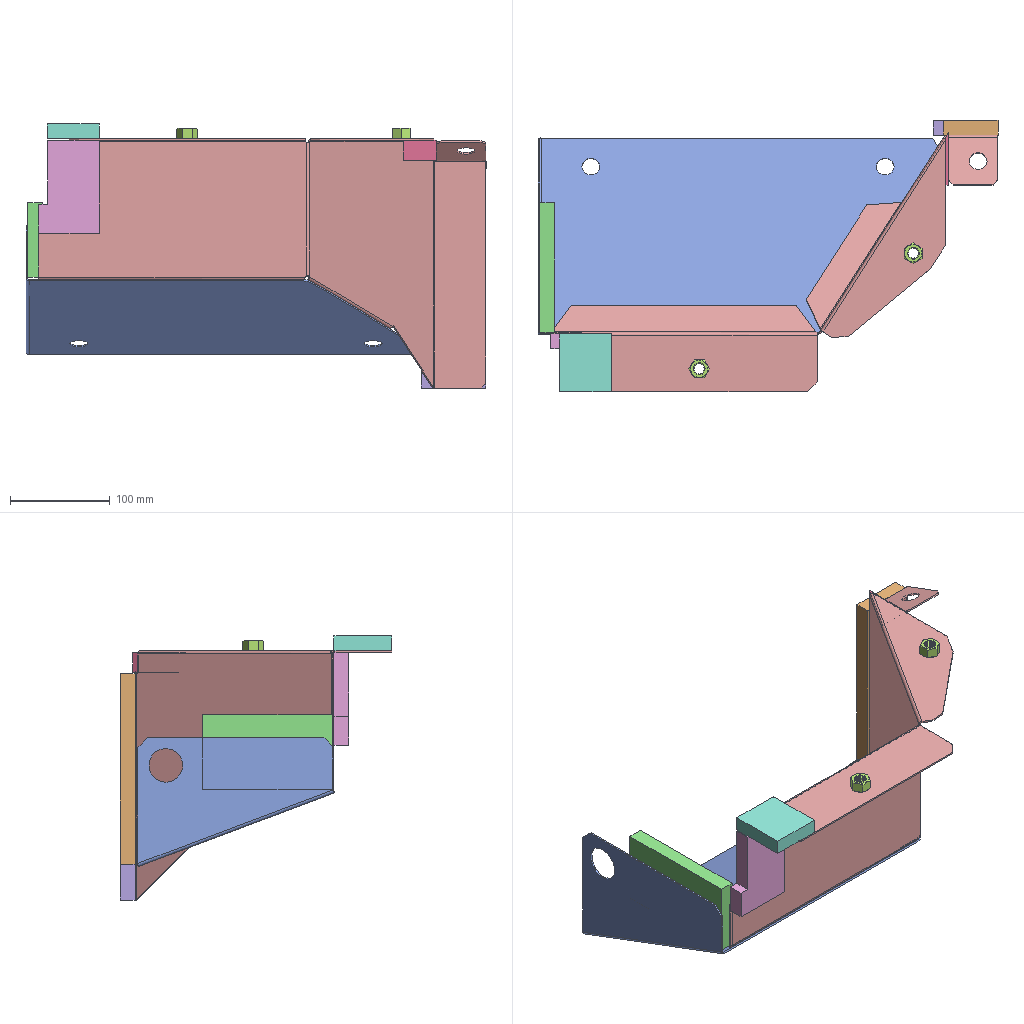Assembly | SolidWorks | 10 different items | 11 placed | box 461 x 272 x 265 mm
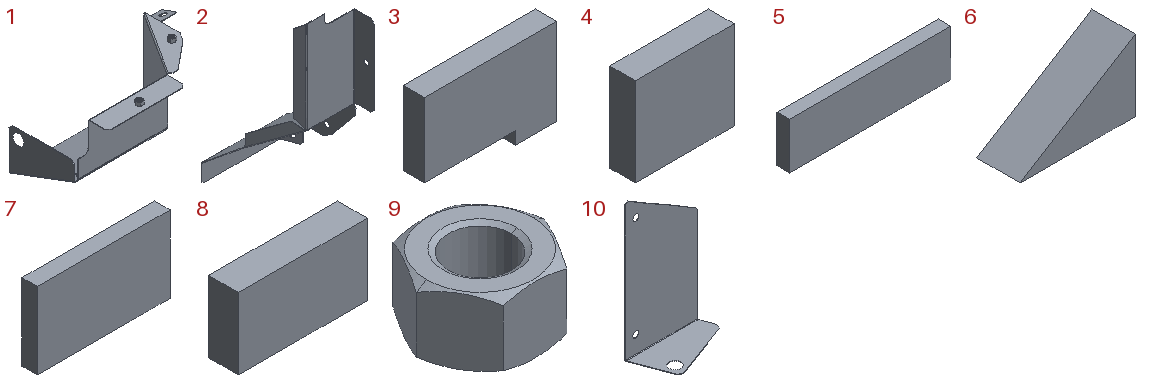Parts list (item | name | quantity | parent item | size | volume | features):
1 | (subassembly) | x1 | - | 461.2 x 257.358 x 260.639 mm | 345314 mm3 | -
2 | - | x1 | in 1 | 249.839 x 257.358 x 448.59 mm | 199881 mm3 | features SM3dBend 7, FlatPattern 1, SMBaseFlange 1, SheetMetal 1
3 | - | x1 | - | 93 x 15 x 61 mm | 76455 mm3 | features FlatPattern 1, SMBaseFlange 1, SheetMetal 1
4 | - | x1 | - | 58 x 15 x 52 mm | 45240 mm3 | features FlatPattern 1, SMBaseFlange 1, SheetMetal 1
5 | - | x1 | - | 191 x 15 x 55 mm | 157575 mm3 | features FlatPattern 1, SMBaseFlange 1, SheetMetal 1
6 | - | x1 | - | 53 x 20 x 33 mm | 17490 mm3 | features FlatPattern 1, SMBaseFlange 1, SheetMetal 1
7 | - | x1 | - | 130 x 15 x 75 mm | 146250 mm3 | features FlatPattern 1, SMBaseFlange 1, SheetMetal 1
8 | - | x1 | - | 65 x 15 x 36 mm | 35100 mm3 | features FlatPattern 1, SMBaseFlange 1, SheetMetal 1
9 | - | x2 | in 1 | 27.713 x 24 x 14.8 mm | 5071 mm3 | features RevCut 2, Chamfer 1, Extrusion 1, LPattern 1
10 | - | x1 | in 1 | 225.52 x 117.762 x 400.759 mm | 141425 mm3 | features FlatPattern 1, SM3dBend 1, SMBaseFlange 1, SheetMetal 1
Mates (type | each side: item.copy, entity, surface, feature):
In the top assembly
Coincident | 2.1 face plane Base-Flange1 | 3.1 face plane Base-Flange1 | 3 times
Coincident | 2.1 face plane Base-Flange1 | 4.1 face plane Base-Flange1 | 2 times
DistanceDim | 4.1 face plane Base-Flange1 | 2.1 face plane Base-Flange1
Coincident | 2.1 face plane Base-Flange1 | 5.1 face plane Base-Flange1 | 2 times
DistanceDim | 5.1 face plane Base-Flange1 | 2.1 face plane Base-Flange1
Coincident | 2.1 face plane Base-Flange1 | 8.1 face plane Base-Flange1 | 3 times
Coincident | 10.1 face plane Base-Flange1 | 7.1 face plane Base-Flange1
DistanceDim | 7.1 face plane Base-Flange1 | 10.1 face plane Base-Flange1
Coincident | 2.1 face plane Base-Flange1 | 7.1 face plane Base-Flange1
Coincident | 2.1 face plane Base-Flange1 | 6.1 face plane Base-Flange1 | 2 times
In subassembly 1
DistanceDim | 10.2 face plane Base-Flange1 | 2.2 face plane Base-Flange1
Coincident | 2.2 face plane Base-Flange1 | 10.2 face plane Base-Flange1
Coincident | 2.2 edge | 10.2 face plane Base-Flange1
Concentric | 2.2 face cylinder Base-Flange1 | 9.1 face cone EndChamfer
Coincident | 2.2 face plane Base-Flange1 | 9.1 face plane BaseNut
Concentric | 2.2 face cylinder Base-Flange1 | 9.2 face cone EndChamfer
Coincident | 2.2 face plane Base-Flange1 | 9.2 face plane BaseNut
Parallel | 2.2 face plane Base-Flange1 | 9.2 face plane BaseNut